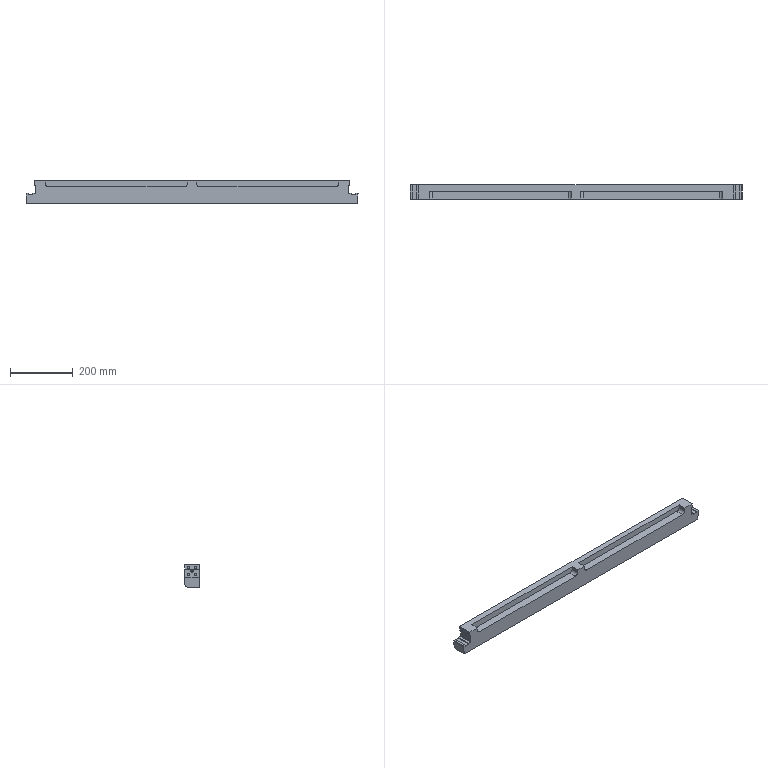NC program | NX | posted with a generic post | part box 1056 x 45 x 72.5 mm
Whole program:
N10 G17 G21 G94 G90
(ZLEVEL_PROFILE , TOOL : D50)
N12 T05 M6
N14 G54
N16 G17 G0 G90 X524.997 Y51.747 B0. C0. S6500 M3
N18 G43 Z43. H5
N20 Z2.5
N22 G94 G1 Z0.573 F2000.
N24 Y22.5
N26 X525. Y22.462
N28 Y-16.872
N30 X524.997 Y-51.747
N32 Z-1.355
N34 X525. Y-16.872
N36 Y22.552
N38 X524.997 Y24.31
N40 Y51.747
N42 Z-3.282
N44 Y24.31
N46 X525. Y22.552
N48 Y-16.872
N50 X524.997 Y-51.747
N52 Z-5.209
N54 X525. Y-16.872
N56 Y22.552
N58 X524.997 Y24.31
N60 Y51.747
N62 Z-7.136
N64 X524.998 Y24.31
N66 X525. Y22.552
N68 Y-16.872
N70 X524.997 Y-51.747
N72 X524.998 Z-9.064
N74 X525. Y-16.872
N76 Y22.552
N78 X524.998 Y24.31
N80 Y51.747
N82 Z-10.991
N84 Y24.31
N86 X525. Y22.552
N88 Y-16.872
N90 X524.998 Y-51.747
N92 Z-12.918
N94 X525. Y-16.872
N96 Y22.552
N98 X524.998 Y51.747
N100 Z-14.845
N102 X525. Y22.552
N104 Y-16.872
N106 X524.998 Y-51.747
N108 Z-16.773
N110 X525. Y-16.872
N112 Y22.552
N114 X524.998 Y51.747
N116 Z-18.7
N118 X525. Y22.552
N120 Y-16.872
N122 X524.998 Y-51.747
N124 Z-20.627
N126 X525. Y-16.872
N128 Y22.552
N130 X524.998 Y51.747
N132 Z-22.555
N134 X525. Y22.552
N136 Y-16.872
N138 X524.998 Y-51.747
N140 Z-24.482
N142 X525. Y-16.872
N144 Y22.552
N146 X524.998 Y51.747
N148 X524.999 Z-26.409
N150 X525. Y22.552
N152 Y-16.872
N154 X524.999 Y-51.747
N156 Z-28.336
N158 X525. Y-16.872
N160 Y22.552
N162 X524.999 Y51.747
N164 Z-30.264
N166 X525. Y22.552
N168 Y-16.872
N170 X524.999 Y-51.747
N172 Z-32.191
N174 X525. Y-16.872
N176 Y22.552
N178 X524.999 Y51.747
N180 Z-34.118
N182 X525. Y22.552
N184 Y-16.872
N186 X524.999 Y-51.747
N188 Z-36.045
N190 X525. Y-16.872
N192 Y22.462
N194 X524.999 Y51.747
N196 Z-37.973
N198 X525. Y22.462
N200 Y-16.872
N202 X524.999 Y-51.747
N204 Z-39.9
N206 X525. Y-16.872
N208 Y22.462
N210 X524.999 Y51.747
N212 G0 Z43.
N214 X-524.997 Y-51.747
N216 Z2.5
N218 G1 Z0.573
N220 X-525. Y-16.872
N222 Y22.525
N224 X-525.002 Y46.572
N226 X-524.997 Y51.747
N228 Z-1.355
N230 X-525.002 Y46.572
N232 X-525. Y22.5
N234 Y-16.872
N236 X-524.997 Y-51.747
N238 Z-3.282
N240 X-525. Y-16.872
N242 Y22.5
N244 X-525.002 Y46.572
N246 X-524.997 Y51.747
N248 Z-5.209
N250 X-525.003 Y46.572
N252 X-525. Y22.5
N254 Y-16.872
N256 X-524.997 Y-51.747
N258 Z-7.136
N260 X-525. Y-16.872
N262 Y22.5
N264 X-525.003 Y46.572
N266 X-524.997 Y51.747
N268 X-524.998 Z-9.064
N270 X-525.003 Y46.572
N272 X-525. Y22.5
N274 Y-16.872
N276 X-524.998 Y-51.747
N278 Z-10.991
N280 X-525. Y-16.872
N282 Y22.5
N284 X-525.003 Y46.572
N286 X-524.998 Y51.747
N288 Z-12.918
N290 X-525.003 Y46.572
N292 X-525. Y22.5
N294 Y-16.872
N296 X-524.998 Y-51.747
N298 Z-14.845
N300 X-525. Y-16.872
N302 Y22.5
N304 X-525.003 Y46.572
N306 X-524.998 Y51.747
N308 Z-16.773
N310 X-525.004 Y46.572
N312 X-525. Y22.5
N314 Y-16.872
N316 X-524.998 Y-51.747
N318 Z-18.7
N320 X-525. Y-16.872
N322 Y22.5
N324 X-525.004 Y46.572
N326 X-524.998 Y51.747
N328 Z-20.627
N330 X-525. Y22.5
N332 Y-16.872
N334 X-524.998 Y-51.747
N336 Z-22.555
N338 X-525. Y-16.872
N340 Y22.5
N342 X-524.998 Y51.747
N344 Z-24.482
N346 X-525. Y22.5
N348 Y-16.872
N350 X-524.998 Y-51.747
N352 X-524.999 Z-26.409
N354 X-525. Y-16.872
N356 Y22.5
N358 X-524.999 Y51.747
N360 Z-28.336
N362 X-525. Y22.5
N364 Y-16.872
N366 X-524.999 Y-51.747
N368 Z-30.264
N370 X-525. Y-16.872
N372 Y22.5
N374 X-524.999 Y51.747
N376 Z-32.191
N378 X-525. Y22.5
N380 Y-16.872
N382 X-524.999 Y-51.747
N384 Z-34.118
N386 X-525. Y-16.872
N388 Y22.5
N390 X-524.999 Y51.747
N392 Z-36.045
N394 X-525. Y22.5
N396 Y-16.872
N398 X-524.999 Y-51.747
N400 Z-37.973
N402 X-525. Y-16.872
N404 Y22.5
N406 X-524.999 Y51.747
N408 Z-39.9
N410 X-525. Y22.5
N412 Y-16.872
N414 X-524.999 Y-51.747
N416 G0 Z43.
(FLOOR_WALL_COPY_COPY , TOOL : D50)
N418 X-525.1 Y-50.7
N420 Z13.
N422 Z-37.
N424 G1 Z-40. F1250.
N426 Y-47.5
N428 Y47.5
N430 Y50.7
N432 Z-37.
N434 G0 Z13.
N436 X525.1
N438 Z-37.
N440 G1 Z-40.
N442 Y47.5
N444 Y-47.5
N446 Y-50.7
N448 Z-37.
N450 G0 Z13.
(ZLEVEL_PROFILE_COPY_2 , TOOL : D50)
N452 Z40.1
N454 X534.357 Y-9.397
N456 Z1.25
N458 G1 X530.431 Y-2.597 F2000.
N460 G3 X526.101 Y-0.097 R5.
N462 G1 X501.833
N464 X499.95 Y-0.1
N466 X-493.924 Y-0.097
N468 X-526.101
N470 G3 X-530.431 Y-2.597 R5.
N472 G1 X-534.356 Y-9.395
N474 G0 Z0.
N476 G1 X-530.431 Y-2.597
N478 G2 X-526.101 Y-0.097 R5.
N480 G1 X-493.87 Y-0.1
N482 X499.95
N484 X501.833 Y-0.097
N486 X526.101
N488 G2 X530.431 Y-2.597 R5.
N490 G1 X534.357 Y-9.397
N492 G0 Z40.1
N494 M5
(ZLEVEL_PROFILE_COPY , TOOL : D12JING)
N496 T21 M6
N498 G54
N500 G17 G0 G90 X514. Y32.905 B0. C0. S6500 M3
N502 G43 Z13. H21
N504 Z-40.775
N506 G94 G1 X513.099 Y30.097 F2000.
N508 G3 X512.499 Y29.058 R1.2
N510 G1 X512.5 Y22.536
N512 Y-22.219
N514 X512.499 Y-29.057
N516 G3 X513.099 Y-30.097 R1.2
N518 G1 X514. Y-32.905
N520 G0 Y-32.906 Z-41.55
N522 G1 X513.1 Y-30.097
N524 G2 X512.5 Y-29.057 R1.2
N526 G1 Y-22.219
N528 Y22.536
N530 Y29.058
N532 G2 X513.1 Y30.097 R1.2
N534 G1 X514. Y32.906
N536 G0 Y32.907 Z-42.325
N538 G1 X513.1 Y30.097
N540 G3 X512.5 Y29.058 R1.2
N542 G1 Y22.465
N544 Y-22.219
N546 Y-29.058
N548 G3 X513.1 Y-30.097 R1.2
N550 G1 X514. Y-32.907
N552 G0 Y-32.908 Z-43.1
N554 G1 X513.101 Y-30.097
N556 G2 X512.501 Y-29.058 R1.2
N558 G1 X512.5 Y-22.219
N560 Y22.465
N562 Y29.058
N564 G2 X513.101 Y30.097 R1.2
N566 G1 X514. Y32.908
N568 G0 Z13.
N570 Y-32.905
N572 Z-40.775
N574 G1 X514.901 Y-30.097
N576 G3 X515.501 Y-29.057 R1.2
N578 G1 X515.5 Y-22.219
N580 Y22.5
N582 X515.557 Y23.333
N584 X515.501 Y23.394
N586 Y29.058
N588 G3 X514.901 Y30.097 R1.2
N590 G1 X514. Y32.905
N592 G0 Y32.906 Z-41.55
N594 G1 X514.9 Y30.097
N596 G2 X515.5 Y29.058 R1.2
N598 G1 Y23.394
N600 X515.557 Y23.333
N602 X515.5 Y22.5
N604 Y-22.219
N606 Y-29.057
N608 G2 X514.9 Y-30.097 R1.2
N610 G1 X514. Y-32.906
N612 G0 Y-32.907 Z-42.325
N614 G1 X514.9 Y-30.097
N616 G3 X515.5 Y-29.058 R1.2
N618 G1 Y-22.219
N620 Y22.5
N622 X515.557 Y23.333
N624 X515.5 Y23.394
N626 Y29.058
N628 G3 X514.9 Y30.097 R1.2
N630 G1 X514. Y32.907
N632 G0 Y32.908 Z-43.1
N634 G1 X514.9 Y30.097
N636 G2 X515.5 Y29.058 R1.2
N638 G1 X515.499 Y23.394
N640 X515.557 Y23.333
N642 X515.5 Y22.465
N644 Y-22.219
N646 X515.499 Y-29.058
N648 G2 X514.899 Y-30.097 R1.2
N650 G1 X514. Y-32.908
N652 G0 Z13.
N654 X-514. Y32.905
N656 Z-40.775
N658 G1 X-514.901 Y30.097
N660 G3 X-515.501 Y29.058 R1.2
N662 G1 X-515.5 Y22.536
N664 Y-22.219
N666 X-515.501 Y-29.057
N668 G3 X-514.901 Y-30.097 R1.2
N670 G1 X-514. Y-32.905
N672 G0 Y-32.906 Z-41.55
N674 G1 X-514.9 Y-30.097
N676 G2 X-515.5 Y-29.057 R1.2
N678 G1 Y-22.219
N680 Y22.536
N682 Y29.058
N684 G2 X-514.9 Y30.097 R1.2
N686 G1 X-514. Y32.906
N688 G0 Y32.907 Z-42.325
N690 G1 X-514.9 Y30.097
N692 G3 X-515.5 Y29.058 R1.2
N694 G1 Y22.465
N696 Y-22.219
N698 Y-29.058
N700 G3 X-514.9 Y-30.097 R1.2
N702 G1 X-514. Y-32.907
N704 G0 Y-32.908 Z-43.1
N706 G1 X-514.899 Y-30.097
N708 G2 X-515.499 Y-29.058 R1.2
N710 G1 X-515.5 Y-22.219
N712 Y22.465
N714 Y29.058
N716 G2 X-514.899 Y30.097 R1.2
N718 G1 X-514. Y32.908
N720 G0 Z13.
N722 Y-32.905
N724 Z-40.775
N726 G1 X-513.099 Y-30.097
N728 G3 X-512.499 Y-29.057 R1.2
N730 G1 X-512.5 Y-22.219
N732 Y22.5
N734 X-512.443 Y23.333
N736 X-512.499 Y23.394
N738 Y29.058
N740 G3 X-513.099 Y30.097 R1.2
N742 G1 X-514. Y32.905
N744 G0 Y32.906 Z-41.55
N746 G1 X-513.1 Y30.097
N748 G2 X-512.5 Y29.058 R1.2
N750 G1 Y23.394
N752 X-512.443 Y23.333
N754 X-512.5 Y22.5
N756 Y-22.219
N758 Y-29.057
N760 G2 X-513.1 Y-30.097 R1.2
N762 G1 X-514. Y-32.906
N764 G0 Y-32.907 Z-42.325
N766 G1 X-513.1 Y-30.097
N768 G3 X-512.5 Y-29.058 R1.2
N770 G1 Y-22.219
N772 Y22.5
N774 X-512.443 Y23.333
N776 X-512.5 Y23.394
N778 Y29.058
N780 G3 X-513.1 Y30.097 R1.2
N782 G1 X-514. Y32.907
N784 G0 Y32.908 Z-43.1
N786 G1 X-513.1 Y30.097
N788 G2 X-512.5 Y29.058 R1.2
N790 G1 X-512.501 Y23.394
N792 X-512.443 Y23.333
N794 X-512.5 Y22.465
N796 Y-22.219
N798 X-512.501 Y-29.058
N800 G2 X-513.101 Y-30.097 R1.2
N802 G1 X-514. Y-32.908
N804 G0 Z13.
(刀补9 , TOOL : D12JING)
N806 Z19.6
N808 X508.323 Y30.23
N810 Z-13.4
N812 G1 Z-14.4 F1000.
N814 G41 X508.223 D21
N816 X506.891 Y29.995
N818 G3 X505.899 Y28.813 R1.2
N820 G1 X505.9 Y22.514
N822 Y-20.556
N824 X505.899 Y-28.813
N826 G3 X506.891 Y-29.995 R1.2
N828 G1 X508.226 Y-30.23
N830 G40
N832 X508.326
N834 Z-13.4
N836 G0 Z19.6
N838 X-508.323 Y-30.236
N840 Z-13.4
N842 G1 Z-14.4
N844 G41 X-508.223
N846 X-506.887 Y-29.997
N848 G3 X-505.899 Y-28.813 R1.2
N850 G1 X-505.9 Y-28.324
N852 Y-20.556
N854 Y22.5
N856 X-505.89 Y22.845
N858 X-505.9 Y22.861
N860 Y28.324
N862 X-505.899 Y28.813
N864 G3 X-506.887 Y29.997 R1.2
N866 G1 X-508.224 Y30.236
N868 G40
N870 X-508.324
N872 Z-13.4
N874 G0 Z19.6
(刀补9. , TOOL : D12JING)
N876 X513.958 Y-32.769
N878 Z13.
N880 Z-42.1
N882 G1 Z-43.1
N884 G41 X514. Y-32.678
N886 X514.618 Y-30.286
N888 G3 X515.6 Y-29.097 R1.2
N890 G1 X515.598 Y-28.813
N892 Y-22.952
N894 X515.6 Y-21.976
N896 Y22.482
N898 X515.598 Y22.5
N900 X515.618 Y22.966
N902 X515.598 Y22.983
N904 Y28.813
N906 X515.6 Y29.097
N908 G3 X514.618 Y30.286 R1.2
N910 G1 X514. Y32.678
N912 G40
N914 X513.959 Y32.769
N916 Z-42.1
N918 G0 Z13.
N920 X514.041
N922 Z-42.1
N924 G1 Z-43.1
N926 G41 X514. Y32.678
N928 X513.391 Y30.279
N930 G3 X512.4 Y29.097 R1.2
N932 G1 Y22.482
N934 Y-21.976
N936 X512.402 Y-22.952
N938 Y-28.813
N940 X512.4 Y-29.097
N942 G3 X513.382 Y-30.286 R1.2
N944 G1 X514. Y-32.678
N946 G40
N948 X514.041 Y-32.769
N950 Z-42.1
N952 G0 Z13.
N954 X-514.042
N956 Z-42.1
N958 G1 Z-43.1
N960 G41 X-514. Y-32.678
N962 X-513.382 Y-30.286
N964 G3 X-512.4 Y-29.097 R1.2
N966 G1 X-512.402 Y-28.813
N968 Y-22.952
N970 X-512.4 Y-21.976
N972 Y22.482
N974 X-512.402 Y22.5
N976 X-512.382 Y22.966
N978 X-512.402 Y22.983
N980 Y28.813
N982 X-512.4 Y29.097
N984 G3 X-513.382 Y30.286 R1.2
N986 G1 X-514. Y32.678
N988 G40
N990 X-514.041 Y32.769
N992 Z-42.1
N994 G0 Z13.
N996 X-513.959
N998 Z-42.1
N1000 G1 Z-43.1
N1002 G41 X-514. Y32.678
N1004 X-514.609 Y30.279
N1006 G3 X-515.6 Y29.097 R1.2
N1008 G1 Y22.482
N1010 Y-21.976
N1012 X-515.598 Y-22.952
N1014 Y-28.813
N1016 X-515.6 Y-29.097
N1018 G3 X-514.618 Y-30.286 R1.2
N1020 G1 X-514. Y-32.678
N1022 G40
N1024 X-513.959 Y-32.769
N1026 Z-42.1
N1028 G0 Z13.
N1030 M5
(PLANAR_MILL , TOOL : T50H10)
N1032 T23 M6
N1034 G54
N1036 G17 G0 G90 X-532. Y-29.26 B0. C0. S6000 M3
N1038 G43 Z10. H23
N1040 Z-24.4
N1042 G94 G1 X-524.857 Y-23.266 F1250.
N1044 G3 X-524.5 Y-22.5 R1.
N1046 G1 Y22.5
N1048 G3 X-524.857 Y23.266 R1.
N1050 G1 X-532. Y29.26
N1052 Y-29.679 F6000.
N1054 X-524.357 Y-23.266 F1250.
N1056 G3 X-524. Y-22.5 R1.
N1058 G1 Y22.5
N1060 G3 X-524.357 Y23.266 R1.
N1062 G1 X-532. Y29.679
N1064 Y-30.099 F6000.
N1066 X-523.857 Y-23.266 F1250.
N1068 G3 X-523.5 Y-22.5 R1.
N1070 G1 Y22.5
N1072 G3 X-523.857 Y23.266 R1.
N1074 G1 X-532. Y30.099
N1076 Y-30.518 F6000.
N1078 X-523.357 Y-23.266 F1250.
N1080 G3 X-523. Y-22.5 R1.
N1082 G1 Y22.5
N1084 G3 X-523.357 Y23.266 R1.
N1086 G1 X-532. Y30.518
N1088 Y-30.938 F6000.
N1090 X-522.857 Y-23.266 F1250.
N1092 G3 X-522.5 Y-22.5 R1.
N1094 G1 Y22.5
N1096 G3 X-522.857 Y23.266 R1.
N1098 G1 X-532. Y30.938
N1100 Y-31.357 F6000.
N1102 X-522.357 Y-23.266 F1250.
N1104 G3 X-522. Y-22.5 R1.
N1106 G1 Y22.5
N1108 G3 X-522.357 Y23.266 R1.
N1110 G1 X-532. Y31.357
N1112 G0 Y-29.26 Z-32.2
N1114 G1 X-524.857 Y-23.266
N1116 G3 X-524.5 Y-22.5 R1.
N1118 G1 Y22.5
N1120 G3 X-524.857 Y23.266 R1.
N1122 G1 X-532. Y29.26
N1124 Y-29.679 F6000.
N1126 X-524.357 Y-23.266 F1250.
N1128 G3 X-524. Y-22.5 R1.
N1130 G1 Y22.5
N1132 G3 X-524.357 Y23.266 R1.
N1134 G1 X-532. Y29.679
N1136 Y-30.099 F6000.
N1138 X-523.857 Y-23.266 F1250.
N1140 G3 X-523.5 Y-22.5 R1.
N1142 G1 Y22.5
N1144 G3 X-523.857 Y23.266 R1.
N1146 G1 X-532. Y30.099
N1148 Y-30.518 F6000.
N1150 X-523.357 Y-23.266 F1250.
N1152 G3 X-523. Y-22.5 R1.
N1154 G1 Y22.5
N1156 G3 X-523.357 Y23.266 R1.
N1158 G1 X-532. Y30.518
N1160 Y-30.938 F6000.
N1162 X-522.857 Y-23.266 F1250.
N1164 G3 X-522.5 Y-22.5 R1.
N1166 G1 Y22.5
N1168 G3 X-522.857 Y23.266 R1.
N1170 G1 X-532. Y30.938
N1172 Y-31.357 F6000.
N1174 X-522.357 Y-23.266 F1250.
N1176 G3 X-522. Y-22.5 R1.
N1178 G1 Y22.5
N1180 G3 X-522.357 Y23.266 R1.
N1182 G1 X-532. Y31.357
N1184 G0 Y-29.26 Z-40.
N1186 G1 X-524.857 Y-23.266
N1188 G3 X-524.5 Y-22.5 R1.
N1190 G1 Y22.5
N1192 G3 X-524.857 Y23.266 R1.
N1194 G1 X-532. Y29.26
N1196 Y-29.679 F6000.
N1198 X-524.357 Y-23.266 F1250.
N1200 G3 X-524. Y-22.5 R1.
N1202 G1 Y22.5
N1204 G3 X-524.357 Y23.266 R1.
N1206 G1 X-532. Y29.679
N1208 Y-30.099 F6000.
N1210 X-523.857 Y-23.266 F1250.
N1212 G3 X-523.5 Y-22.5 R1.
N1214 G1 Y22.5
N1216 G3 X-523.857 Y23.266 R1.
N1218 G1 X-532. Y30.099
N1220 Y-30.518 F6000.
N1222 X-523.357 Y-23.266 F1250.
N1224 G3 X-523. Y-22.5 R1.
N1226 G1 Y22.5
N1228 G3 X-523.357 Y23.266 R1.
N1230 G1 X-532. Y30.518
N1232 Y-30.938 F6000.
N1234 X-522.857 Y-23.266 F1250.
N1236 G3 X-522.5 Y-22.5 R1.
N1238 G1 Y22.5
N1240 G3 X-522.857 Y23.266 R1.
N1242 G1 X-532. Y30.938
N1244 Y-31.357 F6000.
N1246 X-522.357 Y-23.266 F1250.
N1248 G3 X-522. Y-22.5 R1.
N1250 G1 Y22.5
N1252 G3 X-522.357 Y23.266 R1.
N1254 G1 X-532. Y31.357
N1256 G0 Z10.
N1258 X532. Y29.26
N1260 Z-24.4
N1262 G1 X524.857 Y23.266
N1264 G3 X524.5 Y22.5 R1.
N1266 G1 Y-22.5
N1268 G3 X524.857 Y-23.266 R1.
N1270 G1 X532. Y-29.26
N1272 Y29.679 F6000.
N1274 X524.357 Y23.266 F1250.
N1276 G3 X524. Y22.5 R1.
N1278 G1 Y-22.5
N1280 G3 X524.357 Y-23.266 R1.
N1282 G1 X532. Y-29.679
N1284 Y30.099 F6000.
N1286 X523.857 Y23.266 F1250.
N1288 G3 X523.5 Y22.5 R1.
N1290 G1 Y-22.5
N1292 G3 X523.857 Y-23.266 R1.
N1294 G1 X532. Y-30.099
N1296 Y30.518 F6000.
N1298 X523.357 Y23.266 F1250.
N1300 G3 X523. Y22.5 R1.
N1302 G1 Y-22.5
N1304 G3 X523.357 Y-23.266 R1.
N1306 G1 X532. Y-30.518
N1308 Y30.938 F6000.
N1310 X522.857 Y23.266 F1250.
N1312 G3 X522.5 Y22.5 R1.
N1314 G1 Y-22.5
N1316 G3 X522.857 Y-23.266 R1.
N1318 G1 X532. Y-30.938
N1320 Y31.357 F6000.
N1322 X522.357 Y23.266 F1250.
N1324 G3 X522. Y22.5 R1.
N1326 G1 Y-22.5
N1328 G3 X522.357 Y-23.266 R1.
N1330 G1 X532. Y-31.357
N1332 G0 Y29.26 Z-32.2
N1334 G1 X524.857 Y23.266
N1336 G3 X524.5 Y22.5 R1.
N1338 G1 Y-22.5
N1340 G3 X524.857 Y-23.266 R1.
N1342 G1 X532. Y-29.26
N1344 Y29.679 F6000.
N1346 X524.357 Y23.266 F1250.
N1348 G3 X524. Y22.5 R1.
N1350 G1 Y-22.5
N1352 G3 X524.357 Y-23.266 R1.
N1354 G1 X532. Y-29.679
N1356 Y30.099 F6000.
N1358 X523.857 Y23.266 F1250.
N1360 G3 X523.5 Y22.5 R1.
N1362 G1 Y-22.5
N1364 G3 X523.857 Y-23.266 R1.
N1366 G1 X532. Y-30.099
N1368 Y30.518 F6000.
N1370 X523.357 Y23.266 F1250.
N1372 G3 X523. Y22.5 R1.
N1374 G1 Y-22.5
N1376 G3 X523.357 Y-23.266 R1.
N1378 G1 X532. Y-30.518
N1380 Y30.938 F6000.
N1382 X522.857 Y23.266 F1250.
N1384 G3 X522.5 Y22.5 R1.
N1386 G1 Y-22.5
N1388 G3 X522.857 Y-23.266 R1.
N1390 G1 X532. Y-30.938
N1392 Y31.357 F6000.
N1394 X522.357 Y23.266 F1250.
N1396 G3 X522. Y22.5 R1.
N1398 G1 Y-22.5
N1400 G3 X522.357 Y-23.266 R1.
N1402 G1 X532. Y-31.357
N1404 G0 Y29.26 Z-40.
N1406 G1 X524.857 Y23.266
N1408 G3 X524.5 Y22.5 R1.
N1410 G1 Y-22.5
N1412 G3 X524.857 Y-23.266 R1.
N1414 G1 X532. Y-29.26
N1416 Y29.679 F6000.
N1418 X524.357 Y23.266 F1250.
N1420 G3 X524. Y22.5 R1.
N1422 G1 Y-22.5
N1424 G3 X524.357 Y-23.266 R1.
N1426 G1 X532. Y-29.679
N1428 Y30.099 F6000.
N1430 X523.857 Y23.266 F1250.
N1432 G3 X523.5 Y22.5 R1.
N1434 G1 Y-22.5
N1436 G3 X523.857 Y-23.266 R1.
N1438 G1 X532. Y-30.099
N1440 Y30.518 F6000.
N1442 X523.357 Y23.266 F1250.
N1444 G3 X523. Y22.5 R1.
N1446 G1 Y-22.5
N1448 G3 X523.357 Y-23.266 R1.
N1450 G1 X532. Y-30.518
N1452 Y30.938 F6000.
N1454 X522.857 Y23.266 F1250.
N1456 G3 X522.5 Y22.5 R1.
N1458 G1 Y-22.5
N1460 G3 X522.857 Y-23.266 R1.
N1462 G1 X532. Y-30.938
N1464 Y31.357 F6000.
N1466 X522.357 Y23.266 F1250.
N1468 G3 X522. Y22.5 R1.
N1470 G1 Y-22.5
N1472 G3 X522.357 Y-23.266 R1.
N1474 G1 X532. Y-31.357
N1476 G0 Z10.
N1478 M5
(PLANAR_MILL_1 , TOOL : D10A45)
N1480 T07 M6
N1482 G54
N1484 G17 G0 G90 X-1.732 Y25. B0. C0. S7500 M3
N1486 G43 Z10. H7
N1488 Z2.
N1490 G94 G1 Z-1. F1250.
N1492 X-0.866 Y23.5
N1494 G3 X0. Y23. R1.
N1496 G1 X499.4
N1498 G2 X500.4 Y22. R1.
N1500 G1 Y-22.
N1502 G2 X499.4 Y-23. R1.
N1504 G1 X-499.4
N1506 G2 X-500.4 Y-22. R1.
N1508 G1 Y22.
N1510 G2 X-499.4 Y23. R1.
N1512 G1 X0.
N1514 G3 X0.866 Y23.5 R1.
N1516 G1 X1.732 Y25.
N1518 Z2.
N1520 G0 Z10.
(ZLEVEL_PROFILE_1_COPY_1_COPY_COPY_1_COPY , TOOL : D10A45)
N1522 Z13. S7000
N1524 X518.59 Y-32.02
N1526 Z-40.5
N1528 G1 Z-41.5 F1000.
N1530 X519.725 Y-31.364
N1532 G3 X520.225 Y-30.498 R1.
N1534 G1 X520.224 Y-22.502
N1536 Y22.484
N1538 X520.225 Y30.376
N1540 G3 X519.725 Y31.242 R1.
N1542 G1 X518.543 Y31.924
N1544 Z-40.5
N1546 G0 Z13.
N1548 X509.41 Y32.021
N1550 Z-40.5
N1552 G1 Z-41.5
N1554 X508.275 Y31.366
N1556 G3 X507.775 Y30.5 R1.
N1558 G1 X507.776 Y22.502
N1560 Y-22.484
N1562 X507.775 Y-30.483
N1564 G3 X508.275 Y-31.349 R1.
N1566 G1 X509.417 Y-32.009
N1568 Z-40.5
N1570 G0 Z13.
N1572 X-509.41 Y-32.021
N1574 Z-40.5
N1576 G1 Z-41.5
N1578 X-508.275 Y-31.366
N1580 G3 X-507.775 Y-30.5 R1.
N1582 G1 X-507.776 Y-22.502
N1584 Y22.484
N1586 X-507.775 Y30.483
N1588 G3 X-508.275 Y31.349 R1.
N1590 G1 X-509.417 Y32.009
N1592 Z-40.5
N1594 G0 Z13.
N1596 X-518.588 Y32.021
N1598 Z-40.5
N1600 G1 Z-41.5
N1602 X-519.725 Y31.364
N1604 G3 X-520.225 Y30.498 R1.
N1606 G1 X-520.224 Y22.502
N1608 Y-22.484
N1610 X-520.225 Y-30.376
N1612 G3 X-519.725 Y-31.242 R1.
N1614 G1 X-518.542 Y-31.924
N1616 Z-40.5
N1618 G0 Z13.
N1620 M5
N1622 M2